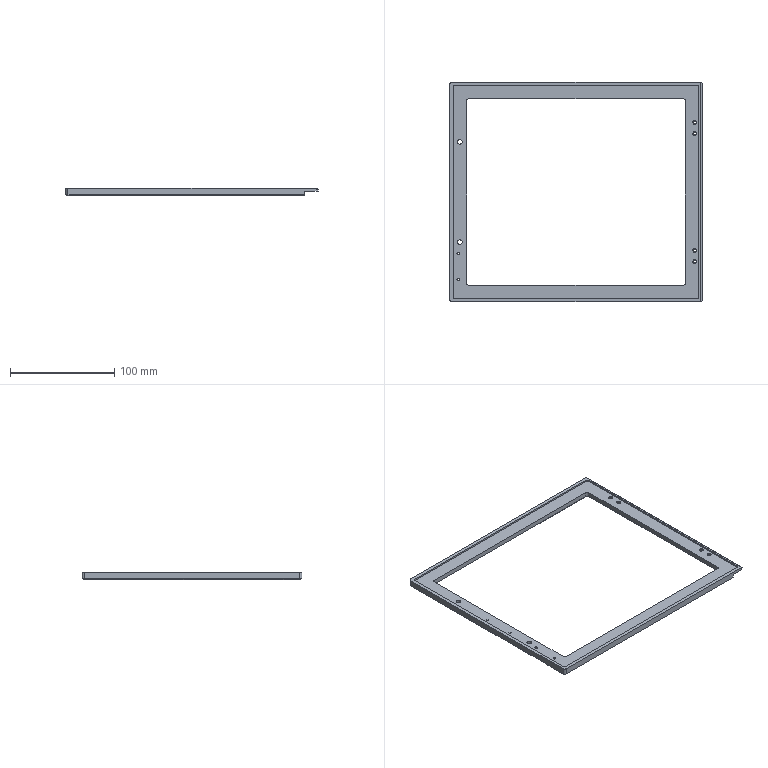NC program | NX | posted with a generic post | part box 241.5 x 210.5 x 7 mm
Lines 416 to 1212 of 3179:
(ZLEVEL_PROFILE_1 , TOOL : D2)
N812 T02 M6
N814 G54
N816 G17 G0 G90 X114.251 Y67.396 S9500 M3
N818 G43 Z30. H2
N820 Z-1.
N822 G94 G1 X114.038 Y67.513 Z-1.013 F1250.
N824 X113.773 Y67.56 Z-1.027
N826 X113.448 Y67.509 Z-1.044
N828 X113.163 Y67.346 Z-1.061
N830 X112.955 Y67.092 Z-1.078
N832 X112.849 Y66.781 Z-1.096
N834 X112.851 Y66.512 Z-1.11
N836 X112.922 Y66.272 Z-1.123
N838 X113.069 Y66.046 Z-1.137
N840 X113.308 Y65.855 Z-1.153
N842 X113.597 Y65.753 Z-1.169
N844 X113.903 Z-1.185
N846 X114.192 Y65.855 Z-1.201
N848 X114.431 Y66.046 Z-1.217
N850 X114.578 Y66.272 Z-1.231
N852 X114.649 Y66.512 Z-1.245
N854 X114.65 Y66.65 Z-1.252
N856 Y66.785 Z-1.259
N858 X114.542 Y67.099 Z-1.276
N860 X114.328 Y67.353 Z-1.294
N862 X114.038 Y67.513 Z-1.311
N864 X113.773 Y67.56 Z-1.325
N866 X113.448 Y67.509 Z-1.342
N868 X113.163 Y67.346 Z-1.36
N870 X112.955 Y67.092 Z-1.377
N872 X112.849 Y66.781 Z-1.394
N874 X112.851 Y66.512 Z-1.408
N876 X112.922 Y66.272 Z-1.421
N878 X113.069 Y66.046 Z-1.435
N880 X113.308 Y65.855 Z-1.451
N882 X113.597 Y65.753 Z-1.467
N884 X113.903 Z-1.483
N886 X114.192 Y65.855 Z-1.499
N888 X114.431 Y66.046 Z-1.516
N890 X114.578 Y66.272 Z-1.53
N892 X114.649 Y66.512 Z-1.543
N894 X114.65 Y66.65 Z-1.55
N896 G3 X113.75 Y67.55 R0.9
N898 X114.65 Y66.65 R-0.9
N900 G1 X114.63 Y66.84 Z-1.553
N902 X114.57 Y67.021 Z-1.557
N904 X114.474 Y67.185 Z-1.56
N906 X114.345 Y67.326 Z-1.563
N908 X114.189 Y67.436 Z-1.567
N910 X114.014 Y67.511 Z-1.57
N912 X113.827 Y67.547 Z-1.573
N914 X113.636 Y67.543 Z-1.577
N916 X113.451 Y67.499 Z-1.58
N918 X113.279 Y67.417 Z-1.583
N920 X113.128 Y67.301 Z-1.587
N922 X113.005 Y67.155 Z-1.59
N924 X112.915 Y66.987 Z-1.593
N926 X112.863 Y66.803 Z-1.597
N928 X112.852 Y66.709 Z-1.598
N930 X112.851 Y66.613 Z-1.6
N932 G3 X114.65 Y66.65 R0.9
N934 G1 X114.63 Y66.84 Z-1.603
N936 X114.57 Y67.021 Z-1.607
N938 X114.474 Y67.185 Z-1.61
N940 X114.345 Y67.326 Z-1.613
N942 X114.189 Y67.436 Z-1.617
N944 X114.014 Y67.511 Z-1.62
N946 X113.827 Y67.547 Z-1.623
N948 X113.636 Y67.543 Z-1.627
N950 X113.451 Y67.499 Z-1.63
N952 X113.279 Y67.417 Z-1.633
N954 X113.128 Y67.301 Z-1.637
N956 X113.005 Y67.155 Z-1.64
N958 X112.915 Y66.987 Z-1.643
N960 X112.863 Y66.803 Z-1.647
N962 X112.852 Y66.709 Z-1.648
N964 X112.851 Y66.613 Z-1.65
N966 G3 X114.65 Y66.65 R0.9
N968 G1 X114.63 Y66.84 Z-1.653
N970 X114.57 Y67.021 Z-1.657
N972 X114.474 Y67.185 Z-1.66
N974 X114.345 Y67.326 Z-1.663
N976 X114.189 Y67.436 Z-1.667
N978 X114.014 Y67.511 Z-1.67
N980 X113.827 Y67.547 Z-1.673
N982 X113.636 Y67.543 Z-1.677
N984 X113.451 Y67.499 Z-1.68
N986 X113.279 Y67.417 Z-1.683
N988 X113.128 Y67.301 Z-1.687
N990 X113.005 Y67.155 Z-1.69
N992 X112.915 Y66.987 Z-1.693
N994 X112.863 Y66.803 Z-1.697
N996 X112.852 Y66.709 Z-1.698
N998 X112.851 Y66.613 Z-1.7
N1000 G3 X114.65 Y66.65 R0.9
N1002 G1 X114.63 Y66.84 Z-1.703
N1004 X114.57 Y67.021 Z-1.707
N1006 X114.474 Y67.185 Z-1.71
N1008 X114.345 Y67.326 Z-1.713
N1010 X114.189 Y67.436 Z-1.717
N1012 X114.014 Y67.511 Z-1.72
N1014 X113.827 Y67.547 Z-1.723
N1016 X113.636 Y67.543 Z-1.727
N1018 X113.451 Y67.499 Z-1.73
N1020 X113.279 Y67.417 Z-1.733
N1022 X113.128 Y67.301 Z-1.737
N1024 X113.005 Y67.155 Z-1.74
N1026 X112.915 Y66.987 Z-1.743
N1028 X112.863 Y66.803 Z-1.747
N1030 X112.852 Y66.709 Z-1.748
N1032 X112.851 Y66.613 Z-1.75
N1034 G3 X114.65 Y66.65 R0.9
N1036 G1 X114.63 Y66.84 Z-1.753
N1038 X114.57 Y67.021 Z-1.757
N1040 X114.474 Y67.185 Z-1.76
N1042 X114.345 Y67.326 Z-1.763
N1044 X114.189 Y67.436 Z-1.767
N1046 X114.014 Y67.511 Z-1.77
N1048 X113.827 Y67.547 Z-1.773
N1050 X113.636 Y67.543 Z-1.777
N1052 X113.451 Y67.499 Z-1.78
N1054 X113.279 Y67.417 Z-1.783
N1056 X113.128 Y67.301 Z-1.787
N1058 X113.005 Y67.155 Z-1.79
N1060 X112.915 Y66.987 Z-1.793
N1062 X112.863 Y66.803 Z-1.797
N1064 X112.852 Y66.709 Z-1.798
N1066 X112.851 Y66.613 Z-1.8
N1068 G3 X114.65 Y66.65 R0.9
N1070 G1 X114.63 Y66.84 Z-1.803
N1072 X114.57 Y67.021 Z-1.807
N1074 X114.474 Y67.185 Z-1.81
N1076 X114.345 Y67.326 Z-1.813
N1078 X114.189 Y67.436 Z-1.817
N1080 X114.014 Y67.511 Z-1.82
N1082 X113.827 Y67.547 Z-1.823
N1084 X113.636 Y67.543 Z-1.827
N1086 X113.451 Y67.499 Z-1.83
N1088 X113.279 Y67.417 Z-1.833
N1090 X113.128 Y67.301 Z-1.837
N1092 X113.005 Y67.155 Z-1.84
N1094 X112.915 Y66.987 Z-1.843
N1096 X112.863 Y66.803 Z-1.847
N1098 X112.852 Y66.709 Z-1.848
N1100 X112.851 Y66.613 Z-1.85
N1102 G3 X114.65 Y66.65 R0.9
N1104 G1 X114.63 Y66.84 Z-1.853
N1106 X114.57 Y67.021 Z-1.857
N1108 X114.474 Y67.185 Z-1.86
N1110 X114.345 Y67.326 Z-1.863
N1112 X114.189 Y67.436 Z-1.867
N1114 X114.014 Y67.511 Z-1.87
N1116 X113.827 Y67.547 Z-1.873
N1118 X113.636 Y67.543 Z-1.877
N1120 X113.451 Y67.499 Z-1.88
N1122 X113.279 Y67.417 Z-1.883
N1124 X113.128 Y67.301 Z-1.887
N1126 X113.005 Y67.155 Z-1.89
N1128 X112.915 Y66.987 Z-1.893
N1130 X112.863 Y66.803 Z-1.897
N1132 X112.852 Y66.709 Z-1.898
N1134 X112.851 Y66.613 Z-1.9
N1136 G3 X114.65 Y66.65 R0.9
N1138 G1 X114.63 Y66.84 Z-1.903
N1140 X114.57 Y67.021 Z-1.907
N1142 X114.474 Y67.185 Z-1.91
N1144 X114.345 Y67.326 Z-1.913
N1146 X114.189 Y67.436 Z-1.917
N1148 X114.014 Y67.511 Z-1.92
N1150 X113.827 Y67.547 Z-1.923
N1152 X113.636 Y67.543 Z-1.927
N1154 X113.451 Y67.499 Z-1.93
N1156 X113.279 Y67.417 Z-1.933
N1158 X113.128 Y67.301 Z-1.937
N1160 X113.005 Y67.155 Z-1.94
N1162 X112.915 Y66.987 Z-1.943
N1164 X112.863 Y66.803 Z-1.947
N1166 X112.852 Y66.709 Z-1.948
N1168 X112.851 Y66.613 Z-1.95
N1170 G3 X114.65 Y66.65 R0.9
N1172 G1 X114.645 Y66.744 Z-1.952
N1174 X114.631 Y66.836 Z-1.953
N1176 X114.573 Y67.014 Z-1.957
N1178 X114.48 Y67.176 Z-1.96
N1180 X114.356 Y67.316 Z-1.963
N1182 X114.205 Y67.427 Z-1.966
N1184 X114.035 Y67.504 Z-1.97
N1186 X113.853 Y67.544 Z-1.973
N1188 X113.666 Y67.546 Z-1.976
N1190 X113.482 Y67.51 Z-1.979
N1192 X113.311 Y67.436 Z-1.983
N1194 X113.158 Y67.328 Z-1.986
N1196 X113.031 Y67.191 Z-1.989
N1198 X112.934 Y67.031 Z-1.992
N1200 X112.873 Y66.854 Z-1.996
N1202 X112.857 Y66.762 Z-1.997
N1204 X112.85 Y66.669 Z-1.999
N1206 Y66.646
N1208 G3 X113.754 Y65.75 R0.9
N1210 X114.65 Y66.65 R0.9
N1212 G1 X114.629 Y66.833 Z-2.002
N1214 X114.571 Y67.006 Z-2.005
N1216 X114.529 Y67.087 Z-2.007
N1218 X114.479 Y67.164 Z-2.009
N1220 X114.412 Y67.244 Z-2.011
N1222 X114.357 Y67.299 Z-2.012
N1224 X114.274 Y67.365 Z-2.014
N1226 X114.211 Y67.406 Z-2.015
N1228 X114.117 Y67.454 Z-2.017
N1230 X114.047 Y67.48 Z-2.018
N1232 X113.945 Y67.508 Z-2.02
N1234 X113.871 Y67.52 Z-2.022
N1236 X113.767 Y67.527 Z-2.023
N1238 X113.692 Y67.524 Z-2.025
N1240 X113.589 Y67.509 Z-2.027
N1242 X113.517 Y67.491 Z-2.028
N1244 X113.419 Y67.455 Z-2.03
N1246 X113.353 Y67.423 Z-2.031
N1248 X113.277 Y67.377 Z-2.033
N1250 X113.206 Y67.323 Z-2.034
N1252 G3 X114.616 Y66.65 R-0.866
N1254 G1 X114.606 Y66.766 Z-2.036
N1256 X114.593 Y66.832 Z-2.038
N1258 X114.562 Y66.936 Z-2.04
N1260 X114.533 Y67.005 Z-2.041
N1262 X114.481 Y67.098 Z-2.043
N1264 X114.438 Y67.16 Z-2.044
N1266 X114.368 Y67.24 Z-2.046
N1268 X114.312 Y67.291 Z-2.047
N1270 X114.227 Y67.355 Z-2.049
N1272 X114.163 Y67.393 Z-2.05
N1274 X114.067 Y67.437 Z-2.052
N1276 X113.996 Y67.46 Z-2.054
N1278 X113.893 Y67.482 Z-2.056
N1280 X113.819 Y67.491 Z-2.057
N1282 X113.714 Z-2.059
N1284 X113.64 Y67.483 Z-2.06
N1286 X113.538 Y67.461 Z-2.062
N1288 X113.468 Y67.438 Z-2.063
N1290 X113.373 Y67.395 Z-2.065
N1292 X113.31 Y67.358 Z-2.067
N1294 X113.238 Y67.306 Z-2.068
N1296 X113.173 Y67.247 Z-2.07
N1298 G3 X114.58 Y66.65 R-0.83
N1300 G1 X114.57 Y66.766 Z-2.072
N1302 X114.557 Y66.832 Z-2.073
N1304 X114.524 Y66.936 Z-2.075
N1306 X114.494 Y67.004 Z-2.076
N1308 X114.44 Y67.096 Z-2.078
N1310 X114.396 Y67.157 Z-2.079
N1312 X114.323 Y67.235 Z-2.081
N1314 X114.266 Y67.284 Z-2.083
N1316 X114.179 Y67.344 Z-2.084
N1318 X114.113 Y67.379 Z-2.086
N1320 X114.015 Y67.418 Z-2.088
N1322 X113.943 Y67.438 Z-2.089
N1324 X113.839 Y67.454 Z-2.091
N1326 X113.765 Y67.458 Z-2.092
N1328 X113.66 Y67.451 Z-2.094
N1330 X113.587 Y67.438 Z-2.095
N1332 X113.487 Y67.409 Z-2.097
N1334 X113.419 Y67.38 Z-2.099
N1336 X113.329 Y67.33 Z-2.101
N1338 X113.269 Y67.287 Z-2.102
N1340 X113.203 Y67.229 Z-2.103
N1342 X113.143 Y67.164 Z-2.105
N1344 G3 X114.545 Y66.65 R-0.795
N1346 G1 X114.534 Y66.766 Z-2.107
N1348 X114.521 Y66.832 Z-2.108
N1350 X114.487 Y66.935 Z-2.11
N1352 X114.455 Y67.003 Z-2.112
N1354 X114.4 Y67.094 Z-2.113
N1356 X114.353 Y67.153 Z-2.115
N1358 X114.278 Y67.229 Z-2.117
N1360 X114.22 Y67.276 Z-2.118
N1362 X114.13 Y67.332 Z-2.12
N1364 X114.062 Y67.364 Z-2.121
N1366 X113.963 Y67.398 Z-2.123
N1368 X113.89 Y67.413 Z-2.124
N1370 X113.785 Y67.423 Z-2.126
N1372 X113.711 Y67.422 Z-2.128
N1374 X113.607 Y67.407 Z-2.129
N1376 X113.536 Y67.389 Z-2.131
N1378 X113.439 Y67.352 Z-2.133
N1380 X113.373 Y67.317 Z-2.134
N1382 X113.288 Y67.259 Z-2.136
N1384 X113.232 Y67.211 Z-2.137
N1386 X113.173 Y67.146 Z-2.139
N1388 X113.12 Y67.075 Z-2.14
N1390 G3 X114.51 Y66.65 R-0.76
N1392 G1 X114.499 Y66.766 Z-2.142
N1394 X114.484 Y66.832 Z-2.144
N1396 X114.449 Y66.935 Z-2.146
N1398 X114.416 Y67.001 Z-2.147
N1400 X114.358 Y67.091 Z-2.149
N1402 X114.31 Y67.149 Z-2.15
N1404 X114.233 Y67.222 Z-2.152
N1406 X114.172 Y67.266 Z-2.153
N1408 X114.08 Y67.318 Z-2.155
N1410 X114.011 Y67.346 Z-2.157
N1412 X113.91 Y67.374 Z-2.158
N1414 X113.836 Y67.385 Z-2.16
N1416 X113.731 Y67.388 Z-2.162
N1418 X113.657 Y67.381 Z-2.163
N1420 X113.555 Y67.359 Z-2.165
N1422 X113.486 Y67.335 Z-2.166
N1424 X113.392 Y67.289 Z-2.168
N1426 X113.331 Y67.249 Z-2.169
N1428 X113.252 Y67.182 Z-2.171
N1430 X113.202 Y67.128 Z-2.173
N1432 X113.149 Y67.058 Z-2.174
N1434 X113.106 Y66.981 Z-2.176
N1436 G3 X114.474 Y66.65 R-0.724
N1438 G1 X114.463 Y66.767 Z-2.178
N1440 X114.448 Y66.832 Z-2.179
N1442 X114.411 Y66.934 Z-2.181
N1444 X114.377 Y67. Z-2.182
N1446 X114.317 Y67.088 Z-2.184
N1448 X114.267 Y67.144 Z-2.185
N1450 X114.187 Y67.214 Z-2.187
N1452 X114.124 Y67.255 Z-2.189
N1454 X114.03 Y67.302 Z-2.191
N1456 X113.959 Y67.327 Z-2.192
N1458 X113.856 Y67.348 Z-2.194
N1460 X113.782 Y67.354 Z-2.195
N1462 X113.677 Y67.349 Z-2.197
N1464 X113.604 Y67.337 Z-2.198
N1466 X113.505 Y67.306 Z-2.2
N1468 X113.438 Y67.275 Z-2.202
N1470 X113.35 Y67.22 Z-2.203
N1472 X113.293 Y67.174 Z-2.205
N1474 X113.222 Y67.099 Z-2.207
N1476 X113.178 Y67.04 Z-2.208
N1478 X113.135 Y66.964 Z-2.21
N1480 X113.102 Y66.883 Z-2.211
N1482 G3 X114.439 Y66.65 R-0.689
N1484 G1 X114.427 Y66.767 Z-2.213
N1486 X114.411 Y66.831 Z-2.214
N1488 X114.373 Y66.933 Z-2.216
N1490 X114.337 Y66.998 Z-2.218
N1492 X114.274 Y67.084 Z-2.219
N1494 X114.222 Y67.138 Z-2.221
N1496 X114.139 Y67.204 Z-2.223
N1498 X114.075 Y67.243 Z-2.224
N1500 X113.978 Y67.285 Z-2.226
N1502 X113.906 Y67.305 Z-2.227
N1504 X113.802 Y67.319 Z-2.229
N1506 X113.728 Z-2.23
N1508 X113.624 Y67.306 Z-2.232
N1510 X113.553 Y67.287 Z-2.234
N1512 X113.457 Y67.247 Z-2.236
N1514 X113.393 Y67.209 Z-2.237
N1516 X113.312 Y67.146 Z-2.239
N1518 X113.261 Y67.093 Z-2.24
N1520 X113.199 Y67.011 Z-2.242
N1522 X113.164 Y66.947 Z-2.243
N1524 X113.131 Y66.866 Z-2.245
N1526 X113.11 Y66.781 Z-2.247
N1528 G3 X114.403 Y66.65 R-0.653
N1530 G1 X114.391 Y66.767 Z-2.249
N1532 X114.375 Y66.831 Z-2.25
N1534 X114.334 Y66.932 Z-2.252
N1536 X114.297 Y66.996 Z-2.253
N1538 X114.231 Y67.08 Z-2.255
N1540 X114.177 Y67.132 Z-2.256
N1542 X114.091 Y67.194 Z-2.258
N1544 X114.025 Y67.229 Z-2.259
N1546 X113.926 Y67.264 Z-2.261
N1548 X113.853 Y67.279 Z-2.263
N1550 X113.748 Y67.286 Z-2.264
N1552 X113.674 Y67.28 Z-2.266
N1554 X113.572 Y67.257 Z-2.268
N1556 X113.503 Y67.231 Z-2.269
N1558 X113.412 Y67.181 Z-2.271
N1560 X113.354 Y67.137 Z-2.272
N1562 X113.281 Y67.064 Z-2.274
N1564 X113.237 Y67.006 Z-2.275
N1566 X113.187 Y66.916 Z-2.277
N1568 X113.161 Y66.848 Z-2.279
N1570 X113.141 Y66.763 Z-2.28
N1572 X113.132 Y66.676 Z-2.282
N1574 G3 X114.368 Y66.65 R-0.618
N1576 G1 X114.355 Y66.767 Z-2.284
N1578 X114.338 Y66.831 Z-2.285
N1580 X114.295 Y66.931 Z-2.287
N1582 X114.256 Y66.993 Z-2.288
N1584 X114.188 Y67.075 Z-2.29
N1586 X114.131 Y67.124 Z-2.292
N1588 X114.042 Y67.182 Z-2.293
N1590 X113.974 Y67.212 Z-2.295
N1592 X113.873 Y67.241 Z-2.297
N1594 X113.799 Y67.25 Z-2.298
N1596 X113.694 Y67.248 Z-2.3
N1598 X113.621 Y67.235 Z-2.301
N1600 X113.523 Y67.202 Z-2.303
N1602 X113.457 Y67.169 Z-2.304
N1604 X113.373 Y67.109 Z-2.306
N1606 X113.32 Y67.058 Z-2.308
N1608 X113.257 Y66.976 Z-2.309
N1610 X113.222 Y66.912 Z-2.311
N1612 X113.187 Y66.816 Z-2.313
N1614 X113.172 Y66.745 Z-2.314
N1616 X113.166 Y66.658 Z-2.316
N1618 X113.173 Y66.572 Z-2.317
N1620 G3 X114.333 Y66.65 R0.583
N1622 G1 X114.319 Y66.767 Z-2.319
N1624 X114.301 Y66.83 Z-2.32
N1626 X114.256 Y66.929 Z-2.322
N1628 X114.215 Y66.991 Z-2.324
N1630 X114.143 Y67.069 Z-2.326
N1632 X114.084 Y67.116 Z-2.327
N1634 X113.992 Y67.168 Z-2.329
N1636 X113.922 Y67.193 Z-2.33
N1638 X113.819 Y67.214 Z-2.332
N1640 X113.745 Y67.217 Z-2.333
N1642 X113.641 Y67.204 Z-2.335
N1644 X113.57 Y67.184 Z-2.337
N1646 X113.476 Y67.14 Z-2.338
N1648 X113.415 Y67.099 Z-2.34
N1650 X113.34 Y67.029 Z-2.342
N1652 X113.295 Y66.971 Z-2.343
N1654 X113.245 Y66.881 Z-2.345
N1656 X113.221 Y66.813 Z-2.346
N1658 X113.202 Y66.713 Z-2.348
N1660 X113.199 Y66.64 Z-2.349
N1662 X113.209 Y66.554 Z-2.351
N1664 X113.233 Y66.471 Z-2.353
N1666 G3 X114.297 Y66.65 R0.547
N1668 G1 X114.283 Y66.767 Z-2.355
N1670 X114.264 Y66.83 Z-2.356
N1672 X114.216 Y66.927 Z-2.358
N1674 X114.173 Y66.987 Z-2.359
N1676 X114.098 Y67.062 Z-2.361
N1678 X114.036 Y67.105 Z-2.362
N1680 X113.941 Y67.151 Z-2.364
N1682 X113.869 Y67.171 Z-2.365
N1684 X113.765 Y67.183 Z-2.367
N1686 X113.691 Y67.178 Z-2.369
N1688 X113.59 Y67.155 Z-2.371
N1690 X113.521 Y67.126 Z-2.372
N1692 X113.434 Y67.071 Z-2.374
N1694 X113.379 Y67.022 Z-2.375
N1696 X113.316 Y66.941 Z-2.377
N1698 X113.28 Y66.877 Z-2.378
N1700 X113.247 Y66.781 Z-2.38
N1702 X113.235 Y66.709 Z-2.382
N1704 Y66.608 Z-2.383
N1706 X113.247 Y66.537 Z-2.385
N1708 X113.275 Y66.455 Z-2.386
N1710 X113.316 Y66.379 Z-2.388
N1712 X113.33 Y66.357
N1714 G3 X114.262 Y66.65 R0.512
N1716 G1 X114.246 Y66.767 Z-2.39
N1718 X114.226 Y66.829 Z-2.391
N1720 X114.176 Y66.925 Z-2.393
N1722 X114.13 Y66.983 Z-2.394
N1724 X114.051 Y67.054 Z-2.396
N1726 X113.987 Y67.093 Z-2.398
N1728 X113.889 Y67.131 Z-2.399
N1730 X113.816 Y67.145 Z-2.401
N1732 X113.711 Y67.146 Z-2.403
N1734 X113.638 Y67.133 Z-2.404
N1736 X113.541 Y67.098 Z-2.406
N1738 X113.477 Y67.061 Z-2.407
N1740 X113.399 Y66.993 Z-2.409
N1742 X113.353 Y66.936 Z-2.41
N1744 X113.304 Y66.847 Z-2.412
N1746 X113.281 Y66.778 Z-2.414
N1748 X113.266 Y66.677 Z-2.416
N1750 X113.269 Y66.604 Z-2.417
N1752 X113.291 Y66.506 Z-2.419
N1754 X113.319 Y66.44 Z-2.42
N1756 X113.365 Y66.367 Z-2.422
N1758 X113.423 Y66.304 Z-2.423
N1760 G3 X114.227 Y66.65 R0.477
N1762 G1 X114.21 Y66.767 Z-2.425
N1764 X114.189 Y66.829 Z-2.427
N1766 X114.135 Y66.923 Z-2.428
N1768 X114.087 Y66.978 Z-2.43
N1770 X114.004 Y67.044 Z-2.432
N1772 X113.937 Y67.078 Z-2.433
N1774 X113.836 Y67.107 Z-2.435
N1776 X113.762 Y67.114 Z-2.436
N1778 X113.658 Y67.103 Z-2.438
N1780 X113.587 Y67.081 Z-2.439
N1782 X113.496 Y67.032 Z-2.441
N1784 X113.439 Y66.986 Z-2.443
N1786 X113.374 Y66.907 Z-2.444
N1788 X113.339 Y66.843 Z-2.446
N1790 X113.308 Y66.745 Z-2.448
N1792 X113.3 Y66.673 Z-2.449
N1794 X113.308 Y66.572 Z-2.451
N1796 X113.327 Y66.503 Z-2.452
N1798 X113.372 Y66.413 Z-2.454
N1800 X113.416 Y66.357 Z-2.455
N1802 X113.479 Y66.3 Z-2.457
N1804 X113.553 Y66.255 Z-2.459
N1806 G3 X114.191 Y66.65 R0.441
N1808 G1 X114.172 Y66.772 Z-2.461
N1810 X114.147 Y66.834 Z-2.462
N1812 X114.109 Y66.899 Z-2.464
N1814 X114.086 Y66.928
N1816 X114.069 Y66.947 Z-2.465
N1818 X114.031 Y66.981 Z-2.466
N1820 X113.934 Y67.041 Z-2.468
N1822 X113.865 Y67.065 Z-2.469
N1824 X113.757 Y67.079 Z-2.471
N1826 X113.681 Y67.072 Z-2.473
N1828 X113.578 Y67.039 Z-2.475
N1830 X113.512 Y67.001 Z-2.476
N1832 X113.433 Y66.929 Z-2.478
N1834 X113.39 Y66.866 Z-2.48
N1836 X113.349 Y66.769 Z-2.482
N1838 X113.336 Y66.695 Z-2.483
N1840 X113.34 Y66.59 Z-2.485
N1842 X113.359 Y66.518 Z-2.487
N1844 X113.406 Y66.425 Z-2.489
N1846 X113.453 Y66.368 Z-2.49
N1848 X113.521 Y66.313 Z-2.492
N1850 X113.6 Y66.273 Z-2.494
N1852 G3 X114.156 Y66.65 R0.406
N1854 G1 X114.146 Y66.733 Z-2.496
N1856 X114.134 Y66.773 Z-2.497
N1858 X114.126 Y66.794
N1860 X114.107 Y66.835 Z-2.498
N1862 X114.063 Y66.901 Z-2.5
N1864 X114.036 Y66.929
N1866 X114.018 Y66.946 Z-2.501
N1868 X113.98 Y66.975 Z-2.502
N1870 X113.911 Y67.013 Z-2.503
N1872 X113.875 Y67.026 Z-2.504
N1874 X113.852 Y67.032 Z-2.505
N1876 X113.804 Y67.041 Z-2.506
N1878 X113.727 Y67.042 Z-2.507
N1880 X113.689 Y67.037 Z-2.508
N1882 X113.666 Y67.032 Z-2.509
N1884 X113.619 Y67.018 Z-2.51
N1886 X113.551 Y66.984 Z-2.511
N1888 X113.52 Y66.963 Z-2.512
N1890 X113.502 Y66.948 Z-2.513
N1892 X113.468 Y66.914 Z-2.514
N1894 X113.423 Y66.853 Z-2.515
N1896 X113.406 Y66.82 Z-2.516
N1898 X113.396 Y66.799 Z-2.517
N1900 X113.382 Y66.754 Z-2.518
N1902 X113.37 Y66.68 Z-2.519
N1904 Y66.643 Z-2.52
N1906 X113.372 Y66.62
N1908 X113.379 Y66.573 Z-2.522
N1910 X113.403 Y66.503 Z-2.523
N1912 X113.419 Y66.471 Z-2.524
N1914 X113.431 Y66.451
N1916 X113.459 Y66.414 Z-2.525
N1918 X113.49 Y66.382 Z-2.526
N1920 X113.524 Y66.354 Z-2.527
N1922 X113.562 Y66.33 Z-2.528
N1924 X113.602 Y66.31 Z-2.529
N1926 G3 X114.121 Y66.65 R0.371
N1928 G1 X114.109 Y66.735 Z-2.531
N1930 X114.096 Y66.774 Z-2.532
N1932 X114.087 Y66.796 Z-2.533
N1934 X114.065 Y66.836 Z-2.534
N1936 X114.016 Y66.899 Z-2.536
N1938 X113.987 Y66.926
N1940 X113.967 Y66.941 Z-2.537
N1942 X113.925 Y66.967 Z-2.538
N1944 X113.852 Y66.996 Z-2.54
N1946 X113.814 Y67.004 Z-2.541
N1948 X113.79 Y67.007
N1950 X113.74 Z-2.543
N1952 X113.663 Y66.995 Z-2.544
N1954 X113.627 Y66.983 Z-2.545
N1956 X113.605 Y66.973 Z-2.546
N1958 X113.562 Y66.949 Z-2.547
N1960 X113.503 Y66.9 Z-2.549
N1962 X113.479 Y66.872 Z-2.55
N1964 X113.465 Y66.852
N1966 X113.44 Y66.81 Z-2.551
N1968 X113.415 Y66.739 Z-2.553
N1970 X113.408 Y66.703 Z-2.554
N1972 X113.406 Y66.679 Z-2.555
N1974 Y66.631 Z-2.556
N1976 X113.42 Y66.558 Z-2.558
N1978 X113.433 Y66.523 Z-2.559
N1980 X113.443 Y66.502
N1982 X113.467 Y66.462 Z-2.56
N1984 X113.496 Y66.427 Z-2.561
N1986 X113.528 Y66.396 Z-2.563
N1988 X113.564 Y66.37 Z-2.564
N1990 X113.604 Y66.348 Z-2.565
N1992 G3 X114.085 Y66.65 R0.335
N1994 G1 X114.075 Y66.726 Z-2.567
N1996 X114.063 Y66.762 Z-2.568
N1998 X114.055 Y66.781
N2000 X114.035 Y66.818 Z-2.569
N2002 X113.991 Y66.875 Z-2.571
N2004 X113.965 Y66.899 Z-2.572
N2006 X113.947 Y66.912
N2008 X113.909 Y66.935 Z-2.574
N2010 X113.843 Y66.961 Z-2.575
N2012 X113.809 Y66.969 Z-2.576
N2014 X113.787 Y66.971 Z-2.577
N2016 X113.742 Y66.972 Z-2.578
N2018 X113.673 Y66.961 Z-2.58
N2020 X113.641 Y66.95 Z-2.581
N2022 X113.621 Y66.942
N2024 X113.583 Y66.92 Z-2.582
N2026 X113.529 Y66.876 Z-2.584
N2028 X113.507 Y66.851 Z-2.585
N2030 X113.495 Y66.834 Z-2.586
N2032 X113.473 Y66.796 Z-2.587
N2034 X113.45 Y66.732 Z-2.589
N2036 X113.443 Y66.7
N2038 X113.441 Y66.678 Z-2.59
N2040 X113.442 Y66.636 Z-2.591
N2042 X113.454 Y66.571 Z-2.593
N2044 X113.464 Y66.54 Z-2.594
N2046 X113.473 Y66.521
N2048 X113.495 Y66.484 Z-2.596
N2050 X113.549 Y66.425 Z-2.598
N2052 X113.615 Y66.379 Z-2.6
N2054 G3 X114.053 Y66.65 R0.302
N2056 G1 X114.023 Y66.751 Z-2.603
N2058 X113.997 Y66.81 Z-2.605
N2060 X113.933 Y66.873 Z-2.608
N2062 X113.869 Y66.913 Z-2.61
N2064 X113.78 Y66.931 Z-2.613
N2066 X113.709 Y66.93 Z-2.615
N2068 X113.626 Y66.898 Z-2.618
N2070 X113.568 Y66.858 Z-2.62
N2072 X113.516 Y66.788 Z-2.623
N2074 X113.49 Y66.725 Z-2.625
N2076 X113.484 Y66.638 Z-2.628
N2078 X113.497 Y66.573 Z-2.63
N2080 X113.512 Y66.539 Z-2.632
N2082 X113.53 Y66.507 Z-2.633
N2084 X113.554 Y66.478 Z-2.634
N2086 X113.583 Y66.454 Z-2.635
N2088 G3 X114.007 Y66.65 R0.257
N2090 G1 X113.995 Y66.725 Z-2.638
N2092 X113.981 Y66.759 Z-2.639
N2094 X113.948 Y66.808 Z-2.641
N2096 X113.896 Y66.853 Z-2.644
N2098 X113.847 Y66.879 Z-2.646
N2100 X113.804 Y66.891 Z-2.647
N2102 X113.737 Y66.894 Z-2.65
N2104 X113.706 Y66.888 Z-2.651
N2106 X113.685 Y66.883 Z-2.652
N2108 X113.645 Y66.866 Z-2.653
N2110 X113.592 Y66.828 Z-2.655
N2112 X113.571 Y66.805 Z-2.657
N2114 X113.559 Y66.788
N2116 X113.54 Y66.751 Z-2.659
N2118 X113.523 Y66.688 Z-2.661
N2120 X113.521 Y66.657 Z-2.663
N2122 X113.522 Y66.638
N2124 X113.529 Y66.599 Z-2.665
N2126 X113.541 Y66.563 Z-2.666
N2128 X113.56 Y66.532 Z-2.668
N2130 X113.584 Y66.503 Z-2.669
N2132 X113.613 Y66.478 Z-2.671
N2134 G3 X113.971 Y66.65 R0.221
N2136 G1 X113.955 Y66.724 Z-2.674
N2138 X113.939 Y66.755 Z-2.675
N2140 X113.928 Y66.772 Z-2.676
N2142 X113.902 Y66.802 Z-2.678
N2144 X113.845 Y66.838 Z-2.681
N2146 X113.815 Y66.849 Z-2.682
N2148 X113.794 Y66.854 Z-2.683
N2150 X113.75 Y66.857 Z-2.685
N2152 X113.686 Y66.843 Z-2.688
N2154 X113.658 Y66.829 Z-2.689
N2156 X113.64 Y66.819 Z-2.69
N2158 X113.609 Y66.791 Z-2.692
N2160 X113.575 Y66.738 Z-2.695
N2162 X113.565 Y66.709 Z-2.696
N2164 X113.56 Y66.69 Z-2.697
N2166 X113.558 Y66.65 Z-2.699
N2168 X113.564 Y66.613 Z-2.701
N2170 X113.576 Y66.579 Z-2.703
N2172 X113.594 Y66.548 Z-2.704
N2174 X113.62 Y66.52 Z-2.706
N2176 G3 X113.88 Y66.52 R0.184
N2178 X113.62 Y66.52 R-0.184
N2180 G1 Z-2.206
N2182 G0 Z30.
N2184 X114.251 Y56.736
N2186 Z-1.
N2188 G1 X114.038 Y56.853 Z-1.013
N2190 X113.773 Y56.899 Z-1.027
N2192 X113.451 Y56.849 Z-1.044
N2194 X113.167 Y56.688 Z-1.061
N2196 X112.958 Y56.438 Z-1.078
N2198 X112.851 Y56.13 Z-1.095
N2200 X112.849 Y55.861 Z-1.109
N2202 X112.922 Y55.611 Z-1.123
N2204 X113.069 Y55.386 Z-1.137
N2206 X113.308 Y55.194 Z-1.153
N2208 X113.597 Y55.093 Z-1.169
N2210 X113.903 Z-1.185
N2212 X114.192 Y55.194 Z-1.201
N2214 X114.431 Y55.386 Z-1.217
N2216 X114.578 Y55.611 Z-1.231
N2218 X114.65 Y55.855 Z-1.245
N2220 Y55.996 Z-1.252
N2222 X114.649 Y56.13 Z-1.259
N2224 X114.54 Y56.442 Z-1.276
N2226 X114.327 Y56.694 Z-1.294
N2228 X114.038 Y56.853 Z-1.311
N2230 X113.773 Y56.899 Z-1.325
N2232 X113.451 Y56.849 Z-1.342
N2234 X113.167 Y56.688 Z-1.359
N2236 X112.958 Y56.438 Z-1.376
N2238 X112.851 Y56.13 Z-1.393
N2240 X112.849 Y55.861 Z-1.408
N2242 X112.922 Y55.611 Z-1.421
N2244 X113.069 Y55.386 Z-1.435
N2246 X113.308 Y55.194 Z-1.451
N2248 X113.597 Y55.093 Z-1.467
N2250 X113.903 Z-1.483
N2252 X114.192 Y55.194 Z-1.499
N2254 X114.431 Y55.386 Z-1.516
N2256 X114.578 Y55.611 Z-1.53
N2258 X114.65 Y55.855 Z-1.543
N2260 Y55.99 Z-1.55
N2262 Y55.996
N2264 G3 X113.744 Y56.89 R0.9
N2266 X114.65 Y55.99 R-0.9
N2268 G1 X114.63 Y56.179 Z-1.553
N2270 X114.57 Y56.36 Z-1.557
N2272 X114.474 Y56.525 Z-1.56
N2274 X114.345 Y56.665 Z-1.563
N2276 X114.189 Y56.775 Z-1.567
N2278 X114.014 Y56.85 Z-1.57
N2280 X113.827 Y56.886 Z-1.573
N2282 X113.636 Y56.882 Z-1.577
N2284 X113.451 Y56.839 Z-1.58
N2286 X113.279 Y56.756 Z-1.583
N2288 X113.128 Y56.64 Z-1.587
N2290 X113.005 Y56.494 Z-1.59
N2292 X112.915 Y56.326 Z-1.593
N2294 X112.863 Y56.143 Z-1.597
N2296 X112.852 Y56.048 Z-1.598
N2298 X112.851 Y55.953 Z-1.6
N2300 G3 X114.65 Y55.99 R0.9
N2302 G1 X114.63 Y56.179 Z-1.603
N2304 X114.57 Y56.36 Z-1.607
N2306 X114.474 Y56.525 Z-1.61
N2308 X114.345 Y56.665 Z-1.613
N2310 X114.189 Y56.775 Z-1.617
N2312 X114.014 Y56.85 Z-1.62
N2314 X113.827 Y56.886 Z-1.623
N2316 X113.636 Y56.882 Z-1.627
N2318 X113.451 Y56.839 Z-1.63
N2320 X113.279 Y56.756 Z-1.633
N2322 X113.128 Y56.64 Z-1.637
N2324 X113.005 Y56.494 Z-1.64
N2326 X112.915 Y56.326 Z-1.643
N2328 X112.863 Y56.143 Z-1.647
N2330 X112.852 Y56.048 Z-1.648
N2332 X112.851 Y55.953 Z-1.65
N2334 G3 X114.65 Y55.99 R0.9
N2336 G1 X114.63 Y56.179 Z-1.653
N2338 X114.57 Y56.36 Z-1.657
N2340 X114.474 Y56.525 Z-1.66
N2342 X114.345 Y56.665 Z-1.663
N2344 X114.189 Y56.775 Z-1.667
N2346 X114.014 Y56.85 Z-1.67
N2348 X113.827 Y56.886 Z-1.673
N2350 X113.636 Y56.882 Z-1.677
N2352 X113.451 Y56.839 Z-1.68
N2354 X113.279 Y56.756 Z-1.683
N2356 X113.128 Y56.64 Z-1.687
N2358 X113.005 Y56.494 Z-1.69
N2360 X112.915 Y56.326 Z-1.693
N2362 X112.863 Y56.143 Z-1.697
N2364 X112.852 Y56.048 Z-1.698
N2366 X112.851 Y55.953 Z-1.7
N2368 G3 X114.65 Y55.99 R0.9
N2370 G1 X114.63 Y56.179 Z-1.703
N2372 X114.57 Y56.36 Z-1.707
N2374 X114.474 Y56.525 Z-1.71
N2376 X114.345 Y56.665 Z-1.713
N2378 X114.189 Y56.775 Z-1.717
N2380 X114.014 Y56.85 Z-1.72
N2382 X113.827 Y56.886 Z-1.723
N2384 X113.636 Y56.882 Z-1.727
N2386 X113.451 Y56.839 Z-1.73
N2388 X113.279 Y56.756 Z-1.733
N2390 X113.128 Y56.64 Z-1.737
N2392 X113.005 Y56.494 Z-1.74
N2394 X112.915 Y56.326 Z-1.743
N2396 X112.863 Y56.143 Z-1.747
N2398 X112.852 Y56.048 Z-1.748